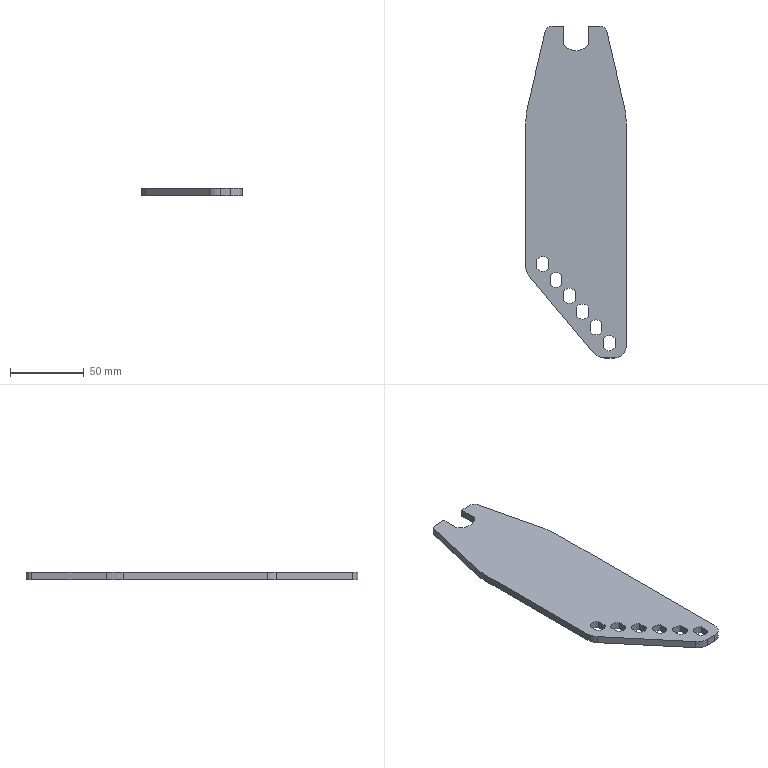Part | SolidWorks | features Fillet 5, ICE 5, Extrusion 1, LPattern 1 | 1 solid | 44 faces | box 68 x 225 x 5 mm | volume 61691 mm3 | plane 24 | cylinder 20 | commonest cylinder face diameters 10.1 x12 10 x2 20 x2 100 x2 16 x1 21 x1
STEP:
#1=CARTESIAN_POINT('',(-26.495,-51.96,5.));
#2=VERTEX_POINT('',#1);
#3=CARTESIAN_POINT('',(-18.495,-51.96,5.));
#4=VERTEX_POINT('',#3);
#5=CARTESIAN_POINT('',(-22.495,-48.877,5.));
#6=DIRECTION('',(0.,0.,1.));
#7=DIRECTION('',(1.,0.,0.));
#8=AXIS2_PLACEMENT_3D('',#5,#6,#7);
#9=CIRCLE('',#8,5.05);
#10=EDGE_CURVE('',#2,#4,#9,.T.);
#11=ORIENTED_EDGE('',*,*,#10,.T.);
#12=CARTESIAN_POINT('',(-18.495,-51.96,0.));
#13=VERTEX_POINT('',#12);
#14=CARTESIAN_POINT('',(-18.495,-51.96,0.));
#15=DIRECTION('',(0.,0.,1.));
#16=VECTOR('',#15,1000.);
#17=LINE('',#14,#16);
#18=EDGE_CURVE('',#13,#4,#17,.T.);
#19=ORIENTED_EDGE('',*,*,#18,.F.);
#20=CARTESIAN_POINT('',(-26.495,-51.96,0.));
#21=VERTEX_POINT('',#20);
#22=CARTESIAN_POINT('',(-22.495,-48.877,0.));
#23=DIRECTION('',(0.,0.,1.));
#24=DIRECTION('',(1.,0.,0.));
#25=AXIS2_PLACEMENT_3D('',#22,#23,#24);
#26=CIRCLE('',#25,5.05);
#27=EDGE_CURVE('',#21,#13,#26,.T.);
#28=ORIENTED_EDGE('',*,*,#27,.F.);
#29=CARTESIAN_POINT('',(-26.495,-51.96,0.));
#30=DIRECTION('',(0.,0.,1.));
#31=VECTOR('',#30,1000.);
#32=LINE('',#29,#31);
#33=EDGE_CURVE('',#21,#2,#32,.T.);
#34=ORIENTED_EDGE('',*,*,#33,.T.);
#35=EDGE_LOOP('',(#11,#19,#28,#34));
#36=FACE_OUTER_BOUND('',#35,.T.);
#37=CARTESIAN_POINT('',(-22.495,-48.877,-3.));
#38=DIRECTION('',(0.,0.,1.));
#39=DIRECTION('',(1.,0.,0.));
#40=AXIS2_PLACEMENT_3D('',#37,#38,#39);
#41=CYLINDRICAL_SURFACE('',#40,5.05);
#42=ADVANCED_FACE('',(#36),#41,.F.);
#43=CARTESIAN_POINT('',(-17.496,-62.684,5.));
#44=VERTEX_POINT('',#43);
#45=CARTESIAN_POINT('',(-9.496,-62.684,5.));
#46=VERTEX_POINT('',#45);
#47=CARTESIAN_POINT('',(-13.496,-59.602,5.));
#48=DIRECTION('',(0.,0.,1.));
#49=DIRECTION('',(1.,0.,0.));
#50=AXIS2_PLACEMENT_3D('',#47,#48,#49);
#51=CIRCLE('',#50,5.05);
#52=EDGE_CURVE('',#44,#46,#51,.T.);
#53=ORIENTED_EDGE('',*,*,#52,.T.);
#54=CARTESIAN_POINT('',(-9.496,-62.684,0.));
#55=VERTEX_POINT('',#54);
#56=CARTESIAN_POINT('',(-9.496,-62.684,0.));
#57=DIRECTION('',(0.,0.,1.));
#58=VECTOR('',#57,1000.);
#59=LINE('',#56,#58);
#60=EDGE_CURVE('',#55,#46,#59,.T.);
#61=ORIENTED_EDGE('',*,*,#60,.F.);
#62=CARTESIAN_POINT('',(-17.496,-62.684,0.));
#63=VERTEX_POINT('',#62);
#64=CARTESIAN_POINT('',(-13.496,-59.602,0.));
#65=DIRECTION('',(0.,0.,1.));
#66=DIRECTION('',(1.,0.,0.));
#67=AXIS2_PLACEMENT_3D('',#64,#65,#66);
#68=CIRCLE('',#67,5.05);
#69=EDGE_CURVE('',#63,#55,#68,.T.);
#70=ORIENTED_EDGE('',*,*,#69,.F.);
#71=CARTESIAN_POINT('',(-17.496,-62.684,0.));
#72=DIRECTION('',(0.,0.,1.));
#73=VECTOR('',#72,1000.);
#74=LINE('',#71,#73);
#75=EDGE_CURVE('',#63,#44,#74,.T.);
#76=ORIENTED_EDGE('',*,*,#75,.T.);
#77=EDGE_LOOP('',(#53,#61,#70,#76));
#78=FACE_OUTER_BOUND('',#77,.T.);
#79=CARTESIAN_POINT('',(-13.496,-59.602,-3.));
#80=DIRECTION('',(0.,0.,1.));
#81=DIRECTION('',(1.,0.,0.));
#82=AXIS2_PLACEMENT_3D('',#79,#80,#81);
#83=CYLINDRICAL_SURFACE('',#82,5.05);
#84=ADVANCED_FACE('',(#78),#83,.F.);
#85=CARTESIAN_POINT('',(-8.497,-73.409,5.));
#86=VERTEX_POINT('',#85);
#87=CARTESIAN_POINT('',(-0.4971,-73.409,5.));
#88=VERTEX_POINT('',#87);
#89=CARTESIAN_POINT('',(-4.497,-70.326,5.));
#90=DIRECTION('',(0.,0.,1.));
#91=DIRECTION('',(1.,0.,0.));
#92=AXIS2_PLACEMENT_3D('',#89,#90,#91);
#93=CIRCLE('',#92,5.05);
#94=EDGE_CURVE('',#86,#88,#93,.T.);
#95=ORIENTED_EDGE('',*,*,#94,.T.);
#96=CARTESIAN_POINT('',(-0.4971,-73.409,0.));
#97=VERTEX_POINT('',#96);
#98=CARTESIAN_POINT('',(-0.4971,-73.409,0.));
#99=DIRECTION('',(0.,0.,1.));
#100=VECTOR('',#99,1000.);
#101=LINE('',#98,#100);
#102=EDGE_CURVE('',#97,#88,#101,.T.);
#103=ORIENTED_EDGE('',*,*,#102,.F.);
#104=CARTESIAN_POINT('',(-8.497,-73.409,0.));
#105=VERTEX_POINT('',#104);
#106=CARTESIAN_POINT('',(-4.497,-70.326,0.));
#107=DIRECTION('',(0.,0.,1.));
#108=DIRECTION('',(1.,0.,0.));
#109=AXIS2_PLACEMENT_3D('',#106,#107,#108);
#110=CIRCLE('',#109,5.05);
#111=EDGE_CURVE('',#105,#97,#110,.T.);
#112=ORIENTED_EDGE('',*,*,#111,.F.);
#113=CARTESIAN_POINT('',(-8.497,-73.409,0.));
#114=DIRECTION('',(0.,0.,1.));
#115=VECTOR('',#114,1000.);
#116=LINE('',#113,#115);
#117=EDGE_CURVE('',#105,#86,#116,.T.);
#118=ORIENTED_EDGE('',*,*,#117,.T.);
#119=EDGE_LOOP('',(#95,#103,#112,#118));
#120=FACE_OUTER_BOUND('',#119,.T.);
#121=CARTESIAN_POINT('',(-4.497,-70.326,-3.));
#122=DIRECTION('',(0.,0.,1.));
#123=DIRECTION('',(1.,0.,0.));
#124=AXIS2_PLACEMENT_3D('',#121,#122,#123);
#125=CYLINDRICAL_SURFACE('',#124,5.05);
#126=ADVANCED_FACE('',(#120),#125,.F.);
#127=CARTESIAN_POINT('',(0.5019,-84.133,5.));
#128=VERTEX_POINT('',#127);
#129=CARTESIAN_POINT('',(8.502,-84.133,5.));
#130=VERTEX_POINT('',#129);
#131=CARTESIAN_POINT('',(4.502,-81.051,5.));
#132=DIRECTION('',(0.,0.,1.));
#133=DIRECTION('',(1.,0.,0.));
#134=AXIS2_PLACEMENT_3D('',#131,#132,#133);
#135=CIRCLE('',#134,5.05);
#136=EDGE_CURVE('',#128,#130,#135,.T.);
#137=ORIENTED_EDGE('',*,*,#136,.T.);
#138=CARTESIAN_POINT('',(8.502,-84.133,0.));
#139=VERTEX_POINT('',#138);
#140=CARTESIAN_POINT('',(8.502,-84.133,0.));
#141=DIRECTION('',(0.,0.,1.));
#142=VECTOR('',#141,1000.);
#143=LINE('',#140,#142);
#144=EDGE_CURVE('',#139,#130,#143,.T.);
#145=ORIENTED_EDGE('',*,*,#144,.F.);
#146=CARTESIAN_POINT('',(0.5019,-84.133,0.));
#147=VERTEX_POINT('',#146);
#148=CARTESIAN_POINT('',(4.502,-81.051,0.));
#149=DIRECTION('',(0.,0.,1.));
#150=DIRECTION('',(1.,0.,0.));
#151=AXIS2_PLACEMENT_3D('',#148,#149,#150);
#152=CIRCLE('',#151,5.05);
#153=EDGE_CURVE('',#147,#139,#152,.T.);
#154=ORIENTED_EDGE('',*,*,#153,.F.);
#155=CARTESIAN_POINT('',(0.5019,-84.133,0.));
#156=DIRECTION('',(0.,0.,1.));
#157=VECTOR('',#156,1000.);
#158=LINE('',#155,#157);
#159=EDGE_CURVE('',#147,#128,#158,.T.);
#160=ORIENTED_EDGE('',*,*,#159,.T.);
#161=EDGE_LOOP('',(#137,#145,#154,#160));
#162=FACE_OUTER_BOUND('',#161,.T.);
#163=CARTESIAN_POINT('',(4.502,-81.051,-3.));
#164=DIRECTION('',(0.,0.,1.));
#165=DIRECTION('',(1.,0.,0.));
#166=AXIS2_PLACEMENT_3D('',#163,#164,#165);
#167=CYLINDRICAL_SURFACE('',#166,5.05);
#168=ADVANCED_FACE('',(#162),#167,.F.);
#169=CARTESIAN_POINT('',(9.501,-94.858,5.));
#170=VERTEX_POINT('',#169);
#171=CARTESIAN_POINT('',(17.501,-94.858,5.));
#172=VERTEX_POINT('',#171);
#173=CARTESIAN_POINT('',(13.501,-91.775,5.));
#174=DIRECTION('',(0.,0.,1.));
#175=DIRECTION('',(1.,0.,0.));
#176=AXIS2_PLACEMENT_3D('',#173,#174,#175);
#177=CIRCLE('',#176,5.05);
#178=EDGE_CURVE('',#170,#172,#177,.T.);
#179=ORIENTED_EDGE('',*,*,#178,.T.);
#180=CARTESIAN_POINT('',(17.501,-94.858,0.));
#181=VERTEX_POINT('',#180);
#182=CARTESIAN_POINT('',(17.501,-94.858,0.));
#183=DIRECTION('',(0.,0.,1.));
#184=VECTOR('',#183,1000.);
#185=LINE('',#182,#184);
#186=EDGE_CURVE('',#181,#172,#185,.T.);
#187=ORIENTED_EDGE('',*,*,#186,.F.);
#188=CARTESIAN_POINT('',(9.501,-94.858,0.));
#189=VERTEX_POINT('',#188);
#190=CARTESIAN_POINT('',(13.501,-91.775,0.));
#191=DIRECTION('',(0.,0.,1.));
#192=DIRECTION('',(1.,0.,0.));
#193=AXIS2_PLACEMENT_3D('',#190,#191,#192);
#194=CIRCLE('',#193,5.05);
#195=EDGE_CURVE('',#189,#181,#194,.T.);
#196=ORIENTED_EDGE('',*,*,#195,.F.);
#197=CARTESIAN_POINT('',(9.501,-94.858,0.));
#198=DIRECTION('',(0.,0.,1.));
#199=VECTOR('',#198,1000.);
#200=LINE('',#197,#199);
#201=EDGE_CURVE('',#189,#170,#200,.T.);
#202=ORIENTED_EDGE('',*,*,#201,.T.);
#203=EDGE_LOOP('',(#179,#187,#196,#202));
#204=FACE_OUTER_BOUND('',#203,.T.);
#205=CARTESIAN_POINT('',(13.501,-91.775,-3.));
#206=DIRECTION('',(0.,0.,1.));
#207=DIRECTION('',(1.,0.,0.));
#208=AXIS2_PLACEMENT_3D('',#205,#206,#207);
#209=CYLINDRICAL_SURFACE('',#208,5.05);
#210=ADVANCED_FACE('',(#204),#209,.F.);
#211=CARTESIAN_POINT('',(18.5,-105.583,5.));
#212=VERTEX_POINT('',#211);
#213=CARTESIAN_POINT('',(26.5,-105.583,5.));
#214=VERTEX_POINT('',#213);
#215=CARTESIAN_POINT('',(22.5,-102.5,5.));
#216=DIRECTION('',(0.,0.,1.));
#217=DIRECTION('',(1.,0.,0.));
#218=AXIS2_PLACEMENT_3D('',#215,#216,#217);
#219=CIRCLE('',#218,5.05);
#220=EDGE_CURVE('',#212,#214,#219,.T.);
#221=ORIENTED_EDGE('',*,*,#220,.T.);
#222=CARTESIAN_POINT('',(26.5,-105.583,0.));
#223=VERTEX_POINT('',#222);
#224=CARTESIAN_POINT('',(26.5,-105.583,0.));
#225=DIRECTION('',(0.,0.,1.));
#226=VECTOR('',#225,1000.);
#227=LINE('',#224,#226);
#228=EDGE_CURVE('',#223,#214,#227,.T.);
#229=ORIENTED_EDGE('',*,*,#228,.F.);
#230=CARTESIAN_POINT('',(18.5,-105.583,0.));
#231=VERTEX_POINT('',#230);
#232=CARTESIAN_POINT('',(22.5,-102.5,0.));
#233=DIRECTION('',(0.,0.,1.));
#234=DIRECTION('',(1.,0.,0.));
#235=AXIS2_PLACEMENT_3D('',#232,#233,#234);
#236=CIRCLE('',#235,5.05);
#237=EDGE_CURVE('',#231,#223,#236,.T.);
#238=ORIENTED_EDGE('',*,*,#237,.F.);
#239=CARTESIAN_POINT('',(18.5,-105.583,0.));
#240=DIRECTION('',(0.,0.,1.));
#241=VECTOR('',#240,1000.);
#242=LINE('',#239,#241);
#243=EDGE_CURVE('',#231,#212,#242,.T.);
#244=ORIENTED_EDGE('',*,*,#243,.T.);
#245=EDGE_LOOP('',(#221,#229,#238,#244));
#246=FACE_OUTER_BOUND('',#245,.T.);
#247=CARTESIAN_POINT('',(22.5,-102.5,-3.));
#248=DIRECTION('',(0.,0.,1.));
#249=DIRECTION('',(1.,0.,0.));
#250=AXIS2_PLACEMENT_3D('',#247,#248,#249);
#251=CYLINDRICAL_SURFACE('',#250,5.05);
#252=ADVANCED_FACE('',(#246),#251,.F.);
#253=CARTESIAN_POINT('',(16.032,112.5,5.));
#254=VERTEX_POINT('',#253);
#255=CARTESIAN_POINT('',(8.5,112.5,5.));
#256=VERTEX_POINT('',#255);
#257=CARTESIAN_POINT('',(-34.,112.5,5.));
#258=DIRECTION('',(-1.,0.,0.));
#259=VECTOR('',#258,1000.);
#260=LINE('',#257,#259);
#261=EDGE_CURVE('',#254,#256,#260,.T.);
#262=ORIENTED_EDGE('',*,*,#261,.F.);
#263=CARTESIAN_POINT('',(16.032,112.5,0.));
#264=VERTEX_POINT('',#263);
#265=CARTESIAN_POINT('',(16.032,112.5,5.));
#266=DIRECTION('',(0.,0.,-1.));
#267=VECTOR('',#266,1000.);
#268=LINE('',#265,#267);
#269=EDGE_CURVE('',#254,#264,#268,.T.);
#270=ORIENTED_EDGE('',*,*,#269,.T.);
#271=CARTESIAN_POINT('',(8.5,112.5,0.));
#272=VERTEX_POINT('',#271);
#273=CARTESIAN_POINT('',(-34.,112.5,0.));
#274=DIRECTION('',(-1.,0.,0.));
#275=VECTOR('',#274,1000.);
#276=LINE('',#273,#275);
#277=EDGE_CURVE('',#264,#272,#276,.T.);
#278=ORIENTED_EDGE('',*,*,#277,.T.);
#279=CARTESIAN_POINT('',(8.5,112.5,-3.));
#280=DIRECTION('',(0.,0.,1.));
#281=VECTOR('',#280,1000.);
#282=LINE('',#279,#281);
#283=EDGE_CURVE('',#272,#256,#282,.T.);
#284=ORIENTED_EDGE('',*,*,#283,.T.);
#285=EDGE_LOOP('',(#262,#270,#278,#284));
#286=FACE_OUTER_BOUND('',#285,.T.);
#287=CARTESIAN_POINT('',(-34.,112.5,5.));
#288=DIRECTION('',(0.,-1.,0.));
#289=DIRECTION('',(0.,0.,-1.));
#290=AXIS2_PLACEMENT_3D('',#287,#288,#289);
#291=PLANE('',#290);
#292=ADVANCED_FACE('',(#286),#291,.F.);
#293=CARTESIAN_POINT('',(34.,-104.5,0.));
#294=VERTEX_POINT('',#293);
#295=CARTESIAN_POINT('',(34.,46.744,0.));
#296=VERTEX_POINT('',#295);
#297=CARTESIAN_POINT('',(34.,112.5,0.));
#298=DIRECTION('',(0.,1.,0.));
#299=VECTOR('',#298,1000.);
#300=LINE('',#297,#299);
#301=EDGE_CURVE('',#294,#296,#300,.T.);
#302=ORIENTED_EDGE('',*,*,#301,.T.);
#303=CARTESIAN_POINT('',(34.,46.744,5.));
#304=VERTEX_POINT('',#303);
#305=CARTESIAN_POINT('',(34.,46.744,5.));
#306=DIRECTION('',(0.,0.,1.));
#307=VECTOR('',#306,1000.);
#308=LINE('',#305,#307);
#309=EDGE_CURVE('',#296,#304,#308,.T.);
#310=ORIENTED_EDGE('',*,*,#309,.T.);
#311=CARTESIAN_POINT('',(34.,-104.5,5.));
#312=VERTEX_POINT('',#311);
#313=CARTESIAN_POINT('',(34.,112.5,5.));
#314=DIRECTION('',(0.,1.,0.));
#315=VECTOR('',#314,1000.);
#316=LINE('',#313,#315);
#317=EDGE_CURVE('',#312,#304,#316,.T.);
#318=ORIENTED_EDGE('',*,*,#317,.F.);
#319=CARTESIAN_POINT('',(34.,-104.5,5.));
#320=DIRECTION('',(0.,0.,-1.));
#321=VECTOR('',#320,1000.);
#322=LINE('',#319,#321);
#323=EDGE_CURVE('',#312,#294,#322,.T.);
#324=ORIENTED_EDGE('',*,*,#323,.T.);
#325=EDGE_LOOP('',(#302,#310,#318,#324));
#326=FACE_OUTER_BOUND('',#325,.T.);
#327=CARTESIAN_POINT('',(34.,112.5,5.));
#328=DIRECTION('',(-1.,0.,0.));
#329=DIRECTION('',(0.,-1.,0.));
#330=AXIS2_PLACEMENT_3D('',#327,#328,#329);
#331=PLANE('',#330);
#332=ADVANCED_FACE('',(#326),#331,.F.);
#333=CARTESIAN_POINT('',(-8.5,112.5,0.));
#334=VERTEX_POINT('',#333);
#335=CARTESIAN_POINT('',(-16.032,112.5,0.));
#336=VERTEX_POINT('',#335);
#337=CARTESIAN_POINT('',(-34.,112.5,0.));
#338=DIRECTION('',(-1.,0.,0.));
#339=VECTOR('',#338,1000.);
#340=LINE('',#337,#339);
#341=EDGE_CURVE('',#334,#336,#340,.T.);
#342=ORIENTED_EDGE('',*,*,#341,.T.);
#343=CARTESIAN_POINT('',(-16.032,112.5,5.));
#344=VERTEX_POINT('',#343);
#345=CARTESIAN_POINT('',(-16.032,112.5,5.));
#346=DIRECTION('',(0.,0.,1.));
#347=VECTOR('',#346,1000.);
#348=LINE('',#345,#347);
#349=EDGE_CURVE('',#336,#344,#348,.T.);
#350=ORIENTED_EDGE('',*,*,#349,.T.);
#351=CARTESIAN_POINT('',(-8.5,112.5,5.));
#352=VERTEX_POINT('',#351);
#353=CARTESIAN_POINT('',(-34.,112.5,5.));
#354=DIRECTION('',(-1.,0.,0.));
#355=VECTOR('',#354,1000.);
#356=LINE('',#353,#355);
#357=EDGE_CURVE('',#352,#344,#356,.T.);
#358=ORIENTED_EDGE('',*,*,#357,.F.);
#359=CARTESIAN_POINT('',(-8.5,112.5,-3.));
#360=DIRECTION('',(0.,0.,1.));
#361=VECTOR('',#360,1000.);
#362=LINE('',#359,#361);
#363=EDGE_CURVE('',#334,#352,#362,.T.);
#364=ORIENTED_EDGE('',*,*,#363,.F.);
#365=EDGE_LOOP('',(#342,#350,#358,#364));
#366=FACE_OUTER_BOUND('',#365,.T.);
#367=CARTESIAN_POINT('',(-34.,112.5,5.));
#368=DIRECTION('',(0.,-1.,0.));
#369=DIRECTION('',(0.,0.,-1.));
#370=AXIS2_PLACEMENT_3D('',#367,#368,#369);
#371=PLANE('',#370);
#372=ADVANCED_FACE('',(#366),#371,.F.);
#373=CARTESIAN_POINT('',(-34.,46.744,5.));
#374=VERTEX_POINT('',#373);
#375=CARTESIAN_POINT('',(-34.,-50.973,5.));
#376=VERTEX_POINT('',#375);
#377=CARTESIAN_POINT('',(-34.,112.5,5.));
#378=DIRECTION('',(0.,-1.,0.));
#379=VECTOR('',#378,1000.);
#380=LINE('',#377,#379);
#381=EDGE_CURVE('',#374,#376,#380,.T.);
#382=ORIENTED_EDGE('',*,*,#381,.F.);
#383=CARTESIAN_POINT('',(-34.,46.744,0.));
#384=VERTEX_POINT('',#383);
#385=CARTESIAN_POINT('',(-34.,46.744,5.));
#386=DIRECTION('',(0.,0.,-1.));
#387=VECTOR('',#386,1000.);
#388=LINE('',#385,#387);
#389=EDGE_CURVE('',#374,#384,#388,.T.);
#390=ORIENTED_EDGE('',*,*,#389,.T.);
#391=CARTESIAN_POINT('',(-34.,-50.973,0.));
#392=VERTEX_POINT('',#391);
#393=CARTESIAN_POINT('',(-34.,112.5,0.));
#394=DIRECTION('',(0.,-1.,0.));
#395=VECTOR('',#394,1000.);
#396=LINE('',#393,#395);
#397=EDGE_CURVE('',#384,#392,#396,.T.);
#398=ORIENTED_EDGE('',*,*,#397,.T.);
#399=CARTESIAN_POINT('',(-34.,-50.973,5.));
#400=DIRECTION('',(0.,0.,1.));
#401=VECTOR('',#400,1000.);
#402=LINE('',#399,#401);
#403=EDGE_CURVE('',#392,#376,#402,.T.);
#404=ORIENTED_EDGE('',*,*,#403,.T.);
#405=EDGE_LOOP('',(#382,#390,#398,#404));
#406=FACE_OUTER_BOUND('',#405,.T.);
#407=CARTESIAN_POINT('',(-34.,112.5,5.));
#408=DIRECTION('',(1.,0.,0.));
#409=DIRECTION('',(0.,1.,0.));
#410=AXIS2_PLACEMENT_3D('',#407,#408,#409);
#411=PLANE('',#410);
#412=ADVANCED_FACE('',(#406),#411,.F.);
#413=CARTESIAN_POINT('',(19.236,-112.5,5.));
#414=VERTEX_POINT('',#413);
#415=CARTESIAN_POINT('',(26.,-112.5,5.));
#416=VERTEX_POINT('',#415);
#417=CARTESIAN_POINT('',(-34.,-112.5,5.));
#418=DIRECTION('',(1.,0.,0.));
#419=VECTOR('',#418,1000.);
#420=LINE('',#417,#419);
#421=EDGE_CURVE('',#414,#416,#420,.T.);
#422=ORIENTED_EDGE('',*,*,#421,.F.);
#423=CARTESIAN_POINT('',(19.236,-112.5,0.));
#424=VERTEX_POINT('',#423);
#425=CARTESIAN_POINT('',(19.236,-112.5,5.));
#426=DIRECTION('',(0.,0.,-1.));
#427=VECTOR('',#426,1000.);
#428=LINE('',#425,#427);
#429=EDGE_CURVE('',#414,#424,#428,.T.);
#430=ORIENTED_EDGE('',*,*,#429,.T.);
#431=CARTESIAN_POINT('',(26.,-112.5,0.));
#432=VERTEX_POINT('',#431);
#433=CARTESIAN_POINT('',(-34.,-112.5,0.));
#434=DIRECTION('',(1.,0.,0.));
#435=VECTOR('',#434,1000.);
#436=LINE('',#433,#435);
#437=EDGE_CURVE('',#424,#432,#436,.T.);
#438=ORIENTED_EDGE('',*,*,#437,.T.);
#439=CARTESIAN_POINT('',(26.,-112.5,5.));
#440=DIRECTION('',(0.,0.,1.));
#441=VECTOR('',#440,1000.);
#442=LINE('',#439,#441);
#443=EDGE_CURVE('',#432,#416,#442,.T.);
#444=ORIENTED_EDGE('',*,*,#443,.T.);
#445=EDGE_LOOP('',(#422,#430,#438,#444));
#446=FACE_OUTER_BOUND('',#445,.T.);
#447=CARTESIAN_POINT('',(-34.,-112.5,5.));
#448=DIRECTION('',(0.,1.,0.));
#449=DIRECTION('',(0.,0.,1.));
#450=AXIS2_PLACEMENT_3D('',#447,#448,#449);
#451=PLANE('',#450);
#452=ADVANCED_FACE('',(#446),#451,.F.);
#453=ORIENTED_EDGE('',*,*,#317,.T.);
#454=CARTESIAN_POINT('',(32.692,58.105,5.));
#455=VERTEX_POINT('',#454);
#456=CARTESIAN_POINT('',(-16.,46.744,5.));
#457=DIRECTION('',(0.,0.,1.));
#458=DIRECTION('',(1.,0.,0.));
#459=AXIS2_PLACEMENT_3D('',#456,#457,#458);
#460=CIRCLE('',#459,50.);
#461=EDGE_CURVE('',#304,#455,#460,.T.);
#462=ORIENTED_EDGE('',*,*,#461,.T.);
#463=CARTESIAN_POINT('',(20.902,108.636,5.));
#464=VERTEX_POINT('',#463);
#465=CARTESIAN_POINT('',(20.,112.5,5.));
#466=DIRECTION('',(0.2272,-0.9738,0.));
#467=VECTOR('',#466,1000.);
#468=LINE('',#465,#467);
#469=EDGE_CURVE('',#464,#455,#468,.T.);
#470=ORIENTED_EDGE('',*,*,#469,.F.);
#471=CARTESIAN_POINT('',(16.032,107.5,5.));
#472=DIRECTION('',(0.,0.,1.));
#473=DIRECTION('',(1.,0.,0.));
#474=AXIS2_PLACEMENT_3D('',#471,#472,#473);
#475=CIRCLE('',#474,5.);
#476=EDGE_CURVE('',#464,#254,#475,.T.);
#477=ORIENTED_EDGE('',*,*,#476,.T.);
#478=ORIENTED_EDGE('',*,*,#261,.T.);
#479=CARTESIAN_POINT('',(8.5,100.171,5.));
#480=VERTEX_POINT('',#479);
#481=CARTESIAN_POINT('',(8.5,112.5,5.));
#482=DIRECTION('',(0.,1.,0.));
#483=VECTOR('',#482,1000.);
#484=LINE('',#481,#483);
#485=EDGE_CURVE('',#480,#256,#484,.T.);
#486=ORIENTED_EDGE('',*,*,#485,.F.);
#487=CARTESIAN_POINT('',(-8.5,100.171,5.));
#488=VERTEX_POINT('',#487);
#489=CARTESIAN_POINT('',(0.,106.336,5.));
#490=DIRECTION('',(0.,0.,1.));
#491=DIRECTION('',(1.,0.,0.));
#492=AXIS2_PLACEMENT_3D('',#489,#490,#491);
#493=CIRCLE('',#492,10.5);
#494=EDGE_CURVE('',#488,#480,#493,.T.);
#495=ORIENTED_EDGE('',*,*,#494,.F.);
#496=CARTESIAN_POINT('',(-8.5,112.5,5.));
#497=DIRECTION('',(0.,-1.,0.));
#498=VECTOR('',#497,1000.);
#499=LINE('',#496,#498);
#500=EDGE_CURVE('',#352,#488,#499,.T.);
#501=ORIENTED_EDGE('',*,*,#500,.F.);
#502=ORIENTED_EDGE('',*,*,#357,.T.);
#503=CARTESIAN_POINT('',(-20.902,108.636,5.));
#504=VERTEX_POINT('',#503);
#505=CARTESIAN_POINT('',(-16.032,107.5,5.));
#506=DIRECTION('',(0.,0.,1.));
#507=DIRECTION('',(1.,0.,0.));
#508=AXIS2_PLACEMENT_3D('',#505,#506,#507);
#509=CIRCLE('',#508,5.);
#510=EDGE_CURVE('',#344,#504,#509,.T.);
#511=ORIENTED_EDGE('',*,*,#510,.T.);
#512=CARTESIAN_POINT('',(-32.692,58.105,5.));
#513=VERTEX_POINT('',#512);
#514=CARTESIAN_POINT('',(-20.,112.5,5.));
#515=DIRECTION('',(0.2272,0.9738,0.));
#516=VECTOR('',#515,1000.);
#517=LINE('',#514,#516);
#518=EDGE_CURVE('',#513,#504,#517,.T.);
#519=ORIENTED_EDGE('',*,*,#518,.F.);
#520=CARTESIAN_POINT('',(16.,46.744,5.));
#521=DIRECTION('',(0.,0.,1.));
#522=DIRECTION('',(1.,0.,0.));
#523=AXIS2_PLACEMENT_3D('',#520,#521,#522);
#524=CIRCLE('',#523,50.);
#525=EDGE_CURVE('',#513,#374,#524,.T.);
#526=ORIENTED_EDGE('',*,*,#525,.T.);
#527=ORIENTED_EDGE('',*,*,#381,.T.);
#528=CARTESIAN_POINT('',(-31.66,-57.401,5.));
#529=VERTEX_POINT('',#528);
#530=CARTESIAN_POINT('',(-24.,-50.973,5.));
#531=DIRECTION('',(0.,0.,1.));
#532=DIRECTION('',(1.,0.,0.));
#533=AXIS2_PLACEMENT_3D('',#530,#531,#532);
#534=CIRCLE('',#533,10.);
#535=EDGE_CURVE('',#376,#529,#534,.T.);
#536=ORIENTED_EDGE('',*,*,#535,.T.);
#537=CARTESIAN_POINT('',(11.576,-108.928,5.));
#538=VERTEX_POINT('',#537);
#539=CARTESIAN_POINT('',(14.573,-112.5,5.));
#540=DIRECTION('',(-0.6428,0.766,0.));
#541=VECTOR('',#540,1000.);
#542=LINE('',#539,#541);
#543=EDGE_CURVE('',#538,#529,#542,.T.);
#544=ORIENTED_EDGE('',*,*,#543,.F.);
#545=CARTESIAN_POINT('',(19.236,-102.5,5.));
#546=DIRECTION('',(0.,0.,1.));
#547=DIRECTION('',(1.,0.,0.));
#548=AXIS2_PLACEMENT_3D('',#545,#546,#547);
#549=CIRCLE('',#548,10.);
#550=EDGE_CURVE('',#538,#414,#549,.T.);
#551=ORIENTED_EDGE('',*,*,#550,.T.);
#552=ORIENTED_EDGE('',*,*,#421,.T.);
#553=CARTESIAN_POINT('',(26.,-104.5,5.));
#554=DIRECTION('',(0.,0.,1.));
#555=DIRECTION('',(1.,0.,0.));
#556=AXIS2_PLACEMENT_3D('',#553,#554,#555);
#557=CIRCLE('',#556,8.);
#558=EDGE_CURVE('',#416,#312,#557,.T.);
#559=ORIENTED_EDGE('',*,*,#558,.T.);
#560=EDGE_LOOP('',(#453,#462,#470,#477,#478,#486,#495,#501,#502,#511,#519,#526,#527,#536,#544,#551,#552,#559));
#561=FACE_OUTER_BOUND('',#560,.T.);
#562=ORIENTED_EDGE('',*,*,#220,.F.);
#563=CARTESIAN_POINT('',(18.5,-99.417,5.));
#564=VERTEX_POINT('',#563);
#565=CARTESIAN_POINT('',(18.5,-105.583,5.));
#566=DIRECTION('',(0.,1.,0.));
#567=VECTOR('',#566,1000.);
#568=LINE('',#565,#567);
#569=EDGE_CURVE('',#212,#564,#568,.T.);
#570=ORIENTED_EDGE('',*,*,#569,.T.);
#571=CARTESIAN_POINT('',(26.5,-99.417,5.));
#572=VERTEX_POINT('',#571);
#573=CARTESIAN_POINT('',(22.5,-102.5,5.));
#574=DIRECTION('',(0.,0.,1.));
#575=DIRECTION('',(1.,0.,0.));
#576=AXIS2_PLACEMENT_3D('',#573,#574,#575);
#577=CIRCLE('',#576,5.05);
#578=EDGE_CURVE('',#572,#564,#577,.T.);
#579=ORIENTED_EDGE('',*,*,#578,.F.);
#580=CARTESIAN_POINT('',(26.5,-105.583,5.));
#581=DIRECTION('',(0.,-1.,0.));
#582=VECTOR('',#581,1000.);
#583=LINE('',#580,#582);
#584=EDGE_CURVE('',#572,#214,#583,.T.);
#585=ORIENTED_EDGE('',*,*,#584,.T.);
#586=EDGE_LOOP('',(#562,#570,#579,#585));
#587=FACE_BOUND('',#586,.T.);
#588=ORIENTED_EDGE('',*,*,#178,.F.);
#589=CARTESIAN_POINT('',(9.501,-88.693,5.));
#590=VERTEX_POINT('',#589);
#591=CARTESIAN_POINT('',(9.501,-94.858,5.));
#592=DIRECTION('',(0.,1.,0.));
#593=VECTOR('',#592,1000.);
#594=LINE('',#591,#593);
#595=EDGE_CURVE('',#170,#590,#594,.T.);
#596=ORIENTED_EDGE('',*,*,#595,.T.);
#597=CARTESIAN_POINT('',(17.501,-88.693,5.));
#598=VERTEX_POINT('',#597);
#599=CARTESIAN_POINT('',(13.501,-91.775,5.));
#600=DIRECTION('',(0.,0.,1.));
#601=DIRECTION('',(1.,0.,0.));
#602=AXIS2_PLACEMENT_3D('',#599,#600,#601);
#603=CIRCLE('',#602,5.05);
#604=EDGE_CURVE('',#598,#590,#603,.T.);
#605=ORIENTED_EDGE('',*,*,#604,.F.);
#606=CARTESIAN_POINT('',(17.501,-94.858,5.));
#607=DIRECTION('',(0.,-1.,0.));
#608=VECTOR('',#607,1000.);
#609=LINE('',#606,#608);
#610=EDGE_CURVE('',#598,#172,#609,.T.);
#611=ORIENTED_EDGE('',*,*,#610,.T.);
#612=EDGE_LOOP('',(#588,#596,#605,#611));
#613=FACE_BOUND('',#612,.T.);
#614=ORIENTED_EDGE('',*,*,#136,.F.);
#615=CARTESIAN_POINT('',(0.5019,-77.968,5.));
#616=VERTEX_POINT('',#615);
#617=CARTESIAN_POINT('',(0.5019,-84.133,5.));
#618=DIRECTION('',(0.,1.,0.));
#619=VECTOR('',#618,1000.);
#620=LINE('',#617,#619);
#621=EDGE_CURVE('',#128,#616,#620,.T.);
#622=ORIENTED_EDGE('',*,*,#621,.T.);
#623=CARTESIAN_POINT('',(8.502,-77.968,5.));
#624=VERTEX_POINT('',#623);
#625=CARTESIAN_POINT('',(4.502,-81.051,5.));
#626=DIRECTION('',(0.,0.,1.));
#627=DIRECTION('',(1.,0.,0.));
#628=AXIS2_PLACEMENT_3D('',#625,#626,#627);
#629=CIRCLE('',#628,5.05);
#630=EDGE_CURVE('',#624,#616,#629,.T.);
#631=ORIENTED_EDGE('',*,*,#630,.F.);
#632=CARTESIAN_POINT('',(8.502,-84.133,5.));
#633=DIRECTION('',(0.,-1.,0.));
#634=VECTOR('',#633,1000.);
#635=LINE('',#632,#634);
#636=EDGE_CURVE('',#624,#130,#635,.T.);
#637=ORIENTED_EDGE('',*,*,#636,.T.);
#638=EDGE_LOOP('',(#614,#622,#631,#637));
#639=FACE_BOUND('',#638,.T.);
#640=ORIENTED_EDGE('',*,*,#94,.F.);
#641=CARTESIAN_POINT('',(-8.497,-67.244,5.));
#642=VERTEX_POINT('',#641);
#643=CARTESIAN_POINT('',(-8.497,-73.409,5.));
#644=DIRECTION('',(0.,1.,0.));
#645=VECTOR('',#644,1000.);
#646=LINE('',#643,#645);
#647=EDGE_CURVE('',#86,#642,#646,.T.);
#648=ORIENTED_EDGE('',*,*,#647,.T.);
#649=CARTESIAN_POINT('',(-0.4971,-67.244,5.));
#650=VERTEX_POINT('',#649);
#651=CARTESIAN_POINT('',(-4.497,-70.326,5.));
#652=DIRECTION('',(0.,0.,1.));
#653=DIRECTION('',(1.,0.,0.));
#654=AXIS2_PLACEMENT_3D('',#651,#652,#653);
#655=CIRCLE('',#654,5.05);
#656=EDGE_CURVE('',#650,#642,#655,.T.);
#657=ORIENTED_EDGE('',*,*,#656,.F.);
#658=CARTESIAN_POINT('',(-0.4971,-73.409,5.));
#659=DIRECTION('',(0.,-1.,0.));
#660=VECTOR('',#659,1000.);
#661=LINE('',#658,#660);
#662=EDGE_CURVE('',#650,#88,#661,.T.);
#663=ORIENTED_EDGE('',*,*,#662,.T.);
#664=EDGE_LOOP('',(#640,#648,#657,#663));
#665=FACE_BOUND('',#664,.T.);
#666=ORIENTED_EDGE('',*,*,#52,.F.);
#667=CARTESIAN_POINT('',(-17.496,-56.519,5.));
#668=VERTEX_POINT('',#667);
#669=CARTESIAN_POINT('',(-17.496,-62.684,5.));
#670=DIRECTION('',(0.,1.,0.));
#671=VECTOR('',#670,1000.);
#672=LINE('',#669,#671);
#673=EDGE_CURVE('',#44,#668,#672,.T.);
#674=ORIENTED_EDGE('',*,*,#673,.T.);
#675=CARTESIAN_POINT('',(-9.496,-56.519,5.));
#676=VERTEX_POINT('',#675);
#677=CARTESIAN_POINT('',(-13.496,-59.602,5.));
#678=DIRECTION('',(0.,0.,1.));
#679=DIRECTION('',(1.,0.,0.));
#680=AXIS2_PLACEMENT_3D('',#677,#678,#679);
#681=CIRCLE('',#680,5.05);
#682=EDGE_CURVE('',#676,#668,#681,.T.);
#683=ORIENTED_EDGE('',*,*,#682,.F.);
#684=CARTESIAN_POINT('',(-9.496,-62.684,5.));
#685=DIRECTION('',(0.,-1.,0.));
#686=VECTOR('',#685,1000.);
#687=LINE('',#684,#686);
#688=EDGE_CURVE('',#676,#46,#687,.T.);
#689=ORIENTED_EDGE('',*,*,#688,.T.);
#690=EDGE_LOOP('',(#666,#674,#683,#689));
#691=FACE_BOUND('',#690,.T.);
#692=ORIENTED_EDGE('',*,*,#10,.F.);
#693=CARTESIAN_POINT('',(-26.495,-45.794,5.));
#694=VERTEX_POINT('',#693);
#695=CARTESIAN_POINT('',(-26.495,-51.96,5.));
#696=DIRECTION('',(0.,1.,0.));
#697=VECTOR('',#696,1000.);
#698=LINE('',#695,#697);
#699=EDGE_CURVE('',#2,#694,#698,.T.);
#700=ORIENTED_EDGE('',*,*,#699,.T.);
#701=CARTESIAN_POINT('',(-18.495,-45.794,5.));
#702=VERTEX_POINT('',#701);
#703=CARTESIAN_POINT('',(-22.495,-48.877,5.));
#704=DIRECTION('',(0.,0.,1.));
#705=DIRECTION('',(1.,0.,0.));
#706=AXIS2_PLACEMENT_3D('',#703,#704,#705);
#707=CIRCLE('',#706,5.05);
#708=EDGE_CURVE('',#702,#694,#707,.T.);
#709=ORIENTED_EDGE('',*,*,#708,.F.);
#710=CARTESIAN_POINT('',(-18.495,-51.96,5.));
#711=DIRECTION('',(0.,-1.,0.));
#712=VECTOR('',#711,1000.);
#713=LINE('',#710,#712);
#714=EDGE_CURVE('',#702,#4,#713,.T.);
#715=ORIENTED_EDGE('',*,*,#714,.T.);
#716=EDGE_LOOP('',(#692,#700,#709,#715));
#717=FACE_BOUND('',#716,.T.);
#718=CARTESIAN_POINT('',(0.,0.,5.));
#719=DIRECTION('',(0.,0.,1.));
#720=DIRECTION('',(1.,0.,0.));
#721=AXIS2_PLACEMENT_3D('',#718,#719,#720);
#722=PLANE('',#721);
#723=ADVANCED_FACE('',(#561,#587,#613,#639,#665,#691,#717),#722,.T.);
#724=ORIENTED_EDGE('',*,*,#237,.T.);
#725=CARTESIAN_POINT('',(26.5,-99.417,0.));
#726=VERTEX_POINT('',#725);
#727=CARTESIAN_POINT('',(26.5,-105.583,0.));
#728=DIRECTION('',(0.,-1.,0.));
#729=VECTOR('',#728,1000.);
#730=LINE('',#727,#729);
#731=EDGE_CURVE('',#726,#223,#730,.T.);
#732=ORIENTED_EDGE('',*,*,#731,.F.);
#733=CARTESIAN_POINT('',(18.5,-99.417,0.));
#734=VERTEX_POINT('',#733);
#735=CARTESIAN_POINT('',(22.5,-102.5,0.));
#736=DIRECTION('',(0.,0.,1.));
#737=DIRECTION('',(1.,0.,0.));
#738=AXIS2_PLACEMENT_3D('',#735,#736,#737);
#739=CIRCLE('',#738,5.05);
#740=EDGE_CURVE('',#726,#734,#739,.T.);
#741=ORIENTED_EDGE('',*,*,#740,.T.);
#742=CARTESIAN_POINT('',(18.5,-105.583,0.));
#743=DIRECTION('',(0.,1.,0.));
#744=VECTOR('',#743,1000.);
#745=LINE('',#742,#744);
#746=EDGE_CURVE('',#231,#734,#745,.T.);
#747=ORIENTED_EDGE('',*,*,#746,.F.);
#748=EDGE_LOOP('',(#724,#732,#741,#747));
#749=FACE_BOUND('',#748,.T.);
#750=ORIENTED_EDGE('',*,*,#195,.T.);
#751=CARTESIAN_POINT('',(17.501,-88.693,0.));
#752=VERTEX_POINT('',#751);
#753=CARTESIAN_POINT('',(17.501,-94.858,0.));
#754=DIRECTION('',(0.,-1.,0.));
#755=VECTOR('',#754,1000.);
#756=LINE('',#753,#755);
#757=EDGE_CURVE('',#752,#181,#756,.T.);
#758=ORIENTED_EDGE('',*,*,#757,.F.);
#759=CARTESIAN_POINT('',(9.501,-88.693,0.));
#760=VERTEX_POINT('',#759);
#761=CARTESIAN_POINT('',(13.501,-91.775,0.));
#762=DIRECTION('',(0.,0.,1.));
#763=DIRECTION('',(1.,0.,0.));
#764=AXIS2_PLACEMENT_3D('',#761,#762,#763);
#765=CIRCLE('',#764,5.05);
#766=EDGE_CURVE('',#752,#760,#765,.T.);
#767=ORIENTED_EDGE('',*,*,#766,.T.);
#768=CARTESIAN_POINT('',(9.501,-94.858,0.));
#769=DIRECTION('',(0.,1.,0.));
#770=VECTOR('',#769,1000.);
#771=LINE('',#768,#770);
#772=EDGE_CURVE('',#189,#760,#771,.T.);
#773=ORIENTED_EDGE('',*,*,#772,.F.);
#774=EDGE_LOOP('',(#750,#758,#767,#773));
#775=FACE_BOUND('',#774,.T.);
#776=ORIENTED_EDGE('',*,*,#153,.T.);
#777=CARTESIAN_POINT('',(8.502,-77.968,0.));
#778=VERTEX_POINT('',#777);
#779=CARTESIAN_POINT('',(8.502,-84.133,0.));
#780=DIRECTION('',(0.,-1.,0.));
#781=VECTOR('',#780,1000.);
#782=LINE('',#779,#781);
#783=EDGE_CURVE('',#778,#139,#782,.T.);
#784=ORIENTED_EDGE('',*,*,#783,.F.);
#785=CARTESIAN_POINT('',(0.5019,-77.968,0.));
#786=VERTEX_POINT('',#785);
#787=CARTESIAN_POINT('',(4.502,-81.051,0.));
#788=DIRECTION('',(0.,0.,1.));
#789=DIRECTION('',(1.,0.,0.));
#790=AXIS2_PLACEMENT_3D('',#787,#788,#789);
#791=CIRCLE('',#790,5.05);
#792=EDGE_CURVE('',#778,#786,#791,.T.);
#793=ORIENTED_EDGE('',*,*,#792,.T.);
#794=CARTESIAN_POINT('',(0.5019,-84.133,0.));
#795=DIRECTION('',(0.,1.,0.));
#796=VECTOR('',#795,1000.);
#797=LINE('',#794,#796);
#798=EDGE_CURVE('',#147,#786,#797,.T.);
#799=ORIENTED_EDGE('',*,*,#798,.F.);
#800=EDGE_LOOP('',(#776,#784,#793,#799));
#801=FACE_BOUND('',#800,.T.);
#802=ORIENTED_EDGE('',*,*,#111,.T.);
#803=CARTESIAN_POINT('',(-0.4971,-67.244,0.));
#804=VERTEX_POINT('',#803);
#805=CARTESIAN_POINT('',(-0.4971,-73.409,0.));
#806=DIRECTION('',(0.,-1.,0.));
#807=VECTOR('',#806,1000.);
#808=LINE('',#805,#807);
#809=EDGE_CURVE('',#804,#97,#808,.T.);
#810=ORIENTED_EDGE('',*,*,#809,.F.);
#811=CARTESIAN_POINT('',(-8.497,-67.244,0.));
#812=VERTEX_POINT('',#811);
#813=CARTESIAN_POINT('',(-4.497,-70.326,0.));
#814=DIRECTION('',(0.,0.,1.));
#815=DIRECTION('',(1.,0.,0.));
#816=AXIS2_PLACEMENT_3D('',#813,#814,#815);
#817=CIRCLE('',#816,5.05);
#818=EDGE_CURVE('',#804,#812,#817,.T.);
#819=ORIENTED_EDGE('',*,*,#818,.T.);
#820=CARTESIAN_POINT('',(-8.497,-73.409,0.));
#821=DIRECTION('',(0.,1.,0.));
#822=VECTOR('',#821,1000.);
#823=LINE('',#820,#822);
#824=EDGE_CURVE('',#105,#812,#823,.T.);
#825=ORIENTED_EDGE('',*,*,#824,.F.);
#826=EDGE_LOOP('',(#802,#810,#819,#825));
#827=FACE_BOUND('',#826,.T.);
#828=ORIENTED_EDGE('',*,*,#69,.T.);
#829=CARTESIAN_POINT('',(-9.496,-56.519,0.));
#830=VERTEX_POINT('',#829);
#831=CARTESIAN_POINT('',(-9.496,-62.684,0.));
#832=DIRECTION('',(0.,-1.,0.));
#833=VECTOR('',#832,1000.);
#834=LINE('',#831,#833);
#835=EDGE_CURVE('',#830,#55,#834,.T.);
#836=ORIENTED_EDGE('',*,*,#835,.F.);
#837=CARTESIAN_POINT('',(-17.496,-56.519,0.));
#838=VERTEX_POINT('',#837);
#839=CARTESIAN_POINT('',(-13.496,-59.602,0.));
#840=DIRECTION('',(0.,0.,1.));
#841=DIRECTION('',(1.,0.,0.));
#842=AXIS2_PLACEMENT_3D('',#839,#840,#841);
#843=CIRCLE('',#842,5.05);
#844=EDGE_CURVE('',#830,#838,#843,.T.);
#845=ORIENTED_EDGE('',*,*,#844,.T.);
#846=CARTESIAN_POINT('',(-17.496,-62.684,0.));
#847=DIRECTION('',(0.,1.,0.));
#848=VECTOR('',#847,1000.);
#849=LINE('',#846,#848);
#850=EDGE_CURVE('',#63,#838,#849,.T.);
#851=ORIENTED_EDGE('',*,*,#850,.F.);
#852=EDGE_LOOP('',(#828,#836,#845,#851));
#853=FACE_BOUND('',#852,.T.);
#854=ORIENTED_EDGE('',*,*,#27,.T.);
#855=CARTESIAN_POINT('',(-18.495,-45.794,0.));
#856=VERTEX_POINT('',#855);
#857=CARTESIAN_POINT('',(-18.495,-51.96,0.));
#858=DIRECTION('',(0.,-1.,0.));
#859=VECTOR('',#858,1000.);
#860=LINE('',#857,#859);
#861=EDGE_CURVE('',#856,#13,#860,.T.);
#862=ORIENTED_EDGE('',*,*,#861,.F.);
#863=CARTESIAN_POINT('',(-26.495,-45.794,0.));
#864=VERTEX_POINT('',#863);
#865=CARTESIAN_POINT('',(-22.495,-48.877,0.));
#866=DIRECTION('',(0.,0.,1.));
#867=DIRECTION('',(1.,0.,0.));
#868=AXIS2_PLACEMENT_3D('',#865,#866,#867);
#869=CIRCLE('',#868,5.05);
#870=EDGE_CURVE('',#856,#864,#869,.T.);
#871=ORIENTED_EDGE('',*,*,#870,.T.);
#872=CARTESIAN_POINT('',(-26.495,-51.96,0.));
#873=DIRECTION('',(0.,1.,0.));
#874=VECTOR('',#873,1000.);
#875=LINE('',#872,#874);
#876=EDGE_CURVE('',#21,#864,#875,.T.);
#877=ORIENTED_EDGE('',*,*,#876,.F.);
#878=EDGE_LOOP('',(#854,#862,#871,#877));
#879=FACE_BOUND('',#878,.T.);
#880=CARTESIAN_POINT('',(20.902,108.636,0.));
#881=VERTEX_POINT('',#880);
#882=CARTESIAN_POINT('',(32.692,58.105,0.));
#883=VERTEX_POINT('',#882);
#884=CARTESIAN_POINT('',(20.,112.5,0.));
#885=DIRECTION('',(0.2272,-0.9738,0.));
#886=VECTOR('',#885,1000.);
#887=LINE('',#884,#886);
#888=EDGE_CURVE('',#881,#883,#887,.T.);
#889=ORIENTED_EDGE('',*,*,#888,.T.);
#890=CARTESIAN_POINT('',(-16.,46.744,0.));
#891=DIRECTION('',(0.,0.,-1.));
#892=DIRECTION('',(1.,0.,0.));
#893=AXIS2_PLACEMENT_3D('',#890,#891,#892);
#894=CIRCLE('',#893,50.);
#895=EDGE_CURVE('',#883,#296,#894,.T.);
#896=ORIENTED_EDGE('',*,*,#895,.T.);
#897=ORIENTED_EDGE('',*,*,#301,.F.);
#898=CARTESIAN_POINT('',(26.,-104.5,0.));
#899=DIRECTION('',(0.,0.,-1.));
#900=DIRECTION('',(1.,0.,0.));
#901=AXIS2_PLACEMENT_3D('',#898,#899,#900);
#902=CIRCLE('',#901,8.);
#903=EDGE_CURVE('',#294,#432,#902,.T.);
#904=ORIENTED_EDGE('',*,*,#903,.T.);
#905=ORIENTED_EDGE('',*,*,#437,.F.);
#906=CARTESIAN_POINT('',(11.576,-108.928,0.));
#907=VERTEX_POINT('',#906);
#908=CARTESIAN_POINT('',(19.236,-102.5,0.));
#909=DIRECTION('',(0.,0.,-1.));
#910=DIRECTION('',(1.,0.,0.));
#911=AXIS2_PLACEMENT_3D('',#908,#909,#910);
#912=CIRCLE('',#911,10.);
#913=EDGE_CURVE('',#424,#907,#912,.T.);
#914=ORIENTED_EDGE('',*,*,#913,.T.);
#915=CARTESIAN_POINT('',(-31.66,-57.401,0.));
#916=VERTEX_POINT('',#915);
#917=CARTESIAN_POINT('',(14.573,-112.5,0.));
#918=DIRECTION('',(-0.6428,0.766,0.));
#919=VECTOR('',#918,1000.);
#920=LINE('',#917,#919);
#921=EDGE_CURVE('',#907,#916,#920,.T.);
#922=ORIENTED_EDGE('',*,*,#921,.T.);
#923=CARTESIAN_POINT('',(-24.,-50.973,0.));
#924=DIRECTION('',(0.,0.,-1.));
#925=DIRECTION('',(1.,0.,0.));
#926=AXIS2_PLACEMENT_3D('',#923,#924,#925);
#927=CIRCLE('',#926,10.);
#928=EDGE_CURVE('',#916,#392,#927,.T.);
#929=ORIENTED_EDGE('',*,*,#928,.T.);
#930=ORIENTED_EDGE('',*,*,#397,.F.);
#931=CARTESIAN_POINT('',(-32.692,58.105,0.));
#932=VERTEX_POINT('',#931);
#933=CARTESIAN_POINT('',(16.,46.744,0.));
#934=DIRECTION('',(0.,0.,-1.));
#935=DIRECTION('',(1.,0.,0.));
#936=AXIS2_PLACEMENT_3D('',#933,#934,#935);
#937=CIRCLE('',#936,50.);
#938=EDGE_CURVE('',#384,#932,#937,.T.);
#939=ORIENTED_EDGE('',*,*,#938,.T.);
#940=CARTESIAN_POINT('',(-20.902,108.636,0.));
#941=VERTEX_POINT('',#940);
#942=CARTESIAN_POINT('',(-20.,112.5,0.));
#943=DIRECTION('',(0.2272,0.9738,0.));
#944=VECTOR('',#943,1000.);
#945=LINE('',#942,#944);
#946=EDGE_CURVE('',#932,#941,#945,.T.);
#947=ORIENTED_EDGE('',*,*,#946,.T.);
#948=CARTESIAN_POINT('',(-16.032,107.5,0.));
#949=DIRECTION('',(0.,0.,-1.));
#950=DIRECTION('',(1.,0.,0.));
#951=AXIS2_PLACEMENT_3D('',#948,#949,#950);
#952=CIRCLE('',#951,5.);
#953=EDGE_CURVE('',#941,#336,#952,.T.);
#954=ORIENTED_EDGE('',*,*,#953,.T.);
#955=ORIENTED_EDGE('',*,*,#341,.F.);
#956=CARTESIAN_POINT('',(-8.5,100.171,0.));
#957=VERTEX_POINT('',#956);
#958=CARTESIAN_POINT('',(-8.5,0.,0.));
#959=DIRECTION('',(0.,-1.,0.));
#960=VECTOR('',#959,1000.);
#961=LINE('',#958,#960);
#962=EDGE_CURVE('',#334,#957,#961,.T.);
#963=ORIENTED_EDGE('',*,*,#962,.T.);
#964=CARTESIAN_POINT('',(8.5,100.171,0.));
#965=VERTEX_POINT('',#964);
#966=CARTESIAN_POINT('',(0.,106.336,0.));
#967=DIRECTION('',(0.,0.,1.));
#968=DIRECTION('',(1.,0.,0.));
#969=AXIS2_PLACEMENT_3D('',#966,#967,#968);
#970=CIRCLE('',#969,10.5);
#971=EDGE_CURVE('',#957,#965,#970,.T.);
#972=ORIENTED_EDGE('',*,*,#971,.T.);
#973=CARTESIAN_POINT('',(8.5,0.,0.));
#974=DIRECTION('',(0.,1.,0.));
#975=VECTOR('',#974,1000.);
#976=LINE('',#973,#975);
#977=EDGE_CURVE('',#965,#272,#976,.T.);
#978=ORIENTED_EDGE('',*,*,#977,.T.);
#979=ORIENTED_EDGE('',*,*,#277,.F.);
#980=CARTESIAN_POINT('',(16.032,107.5,0.));
#981=DIRECTION('',(0.,0.,-1.));
#982=DIRECTION('',(1.,0.,0.));
#983=AXIS2_PLACEMENT_3D('',#980,#981,#982);
#984=CIRCLE('',#983,5.);
#985=EDGE_CURVE('',#264,#881,#984,.T.);
#986=ORIENTED_EDGE('',*,*,#985,.T.);
#987=EDGE_LOOP('',(#889,#896,#897,#904,#905,#914,#922,#929,#930,#939,#947,#954,#955,#963,#972,#978,#979,#986));
#988=FACE_OUTER_BOUND('',#987,.T.);
#989=CARTESIAN_POINT('',(0.,0.,0.));
#990=DIRECTION('',(0.,0.,1.));
#991=DIRECTION('',(1.,0.,0.));
#992=AXIS2_PLACEMENT_3D('',#989,#990,#991);
#993=PLANE('',#992);
#994=ADVANCED_FACE('',(#749,#775,#801,#827,#853,#879,#988),#993,.F.);
#995=ORIENTED_EDGE('',*,*,#870,.F.);
#996=CARTESIAN_POINT('',(-18.495,-45.794,0.));
#997=DIRECTION('',(0.,0.,1.));
#998=VECTOR('',#997,1000.);
#999=LINE('',#996,#998);
#1000=EDGE_CURVE('',#856,#702,#999,.T.);
#1001=ORIENTED_EDGE('',*,*,#1000,.T.);
#1002=ORIENTED_EDGE('',*,*,#708,.T.);
#1003=CARTESIAN_POINT('',(-26.495,-45.794,0.));
#1004=DIRECTION('',(0.,0.,1.));
#1005=VECTOR('',#1004,1000.);
#1006=LINE('',#1003,#1005);
#1007=EDGE_CURVE('',#864,#694,#1006,.T.);
#1008=ORIENTED_EDGE('',*,*,#1007,.F.);
#1009=EDGE_LOOP('',(#995,#1001,#1002,#1008));
#1010=FACE_OUTER_BOUND('',#1009,.T.);
#1011=CARTESIAN_POINT('',(-22.495,-48.877,-3.));
#1012=DIRECTION('',(0.,0.,1.));
#1013=DIRECTION('',(1.,0.,0.));
#1014=AXIS2_PLACEMENT_3D('',#1011,#1012,#1013);
#1015=CYLINDRICAL_SURFACE('',#1014,5.05);
#1016=ADVANCED_FACE('',(#1010),#1015,.F.);
#1017=ORIENTED_EDGE('',*,*,#844,.F.);
#1018=CARTESIAN_POINT('',(-9.496,-56.519,0.));
#1019=DIRECTION('',(0.,0.,1.));
#1020=VECTOR('',#1019,1000.);
#1021=LINE('',#1018,#1020);
#1022=EDGE_CURVE('',#830,#676,#1021,.T.);
#1023=ORIENTED_EDGE('',*,*,#1022,.T.);
#1024=ORIENTED_EDGE('',*,*,#682,.T.);
#1025=CARTESIAN_POINT('',(-17.496,-56.519,0.));
#1026=DIRECTION('',(0.,0.,1.));
#1027=VECTOR('',#1026,1000.);
#1028=LINE('',#1025,#1027);
#1029=EDGE_CURVE('',#838,#668,#1028,.T.);
#1030=ORIENTED_EDGE('',*,*,#1029,.F.);
#1031=EDGE_LOOP('',(#1017,#1023,#1024,#1030));
#1032=FACE_OUTER_BOUND('',#1031,.T.);
#1033=CARTESIAN_POINT('',(-13.496,-59.602,-3.));
#1034=DIRECTION('',(0.,0.,1.));
#1035=DIRECTION('',(1.,0.,0.));
#1036=AXIS2_PLACEMENT_3D('',#1033,#1034,#1035);
#1037=CYLINDRICAL_SURFACE('',#1036,5.05);
#1038=ADVANCED_FACE('',(#1032),#1037,.F.);
#1039=ORIENTED_EDGE('',*,*,#818,.F.);
#1040=CARTESIAN_POINT('',(-0.4971,-67.244,0.));
#1041=DIRECTION('',(0.,0.,1.));
#1042=VECTOR('',#1041,1000.);
#1043=LINE('',#1040,#1042);
#1044=EDGE_CURVE('',#804,#650,#1043,.T.);
#1045=ORIENTED_EDGE('',*,*,#1044,.T.);
#1046=ORIENTED_EDGE('',*,*,#656,.T.);
#1047=CARTESIAN_POINT('',(-8.497,-67.244,0.));
#1048=DIRECTION('',(0.,0.,1.));
#1049=VECTOR('',#1048,1000.);
#1050=LINE('',#1047,#1049);
#1051=EDGE_CURVE('',#812,#642,#1050,.T.);
#1052=ORIENTED_EDGE('',*,*,#1051,.F.);
#1053=EDGE_LOOP('',(#1039,#1045,#1046,#1052));
#1054=FACE_OUTER_BOUND('',#1053,.T.);
#1055=CARTESIAN_POINT('',(-4.497,-70.326,-3.));
#1056=DIRECTION('',(0.,0.,1.));
#1057=DIRECTION('',(1.,0.,0.));
#1058=AXIS2_PLACEMENT_3D('',#1055,#1056,#1057);
#1059=CYLINDRICAL_SURFACE('',#1058,5.05);
#1060=ADVANCED_FACE('',(#1054),#1059,.F.);
#1061=ORIENTED_EDGE('',*,*,#792,.F.);
#1062=CARTESIAN_POINT('',(8.502,-77.968,0.));
#1063=DIRECTION('',(0.,0.,1.));
#1064=VECTOR('',#1063,1000.);
#1065=LINE('',#1062,#1064);
#1066=EDGE_CURVE('',#778,#624,#1065,.T.);
#1067=ORIENTED_EDGE('',*,*,#1066,.T.);
#1068=ORIENTED_EDGE('',*,*,#630,.T.);
#1069=CARTESIAN_POINT('',(0.5019,-77.968,0.));
#1070=DIRECTION('',(0.,0.,1.));
#1071=VECTOR('',#1070,1000.);
#1072=LINE('',#1069,#1071);
#1073=EDGE_CURVE('',#786,#616,#1072,.T.);
#1074=ORIENTED_EDGE('',*,*,#1073,.F.);
#1075=EDGE_LOOP('',(#1061,#1067,#1068,#1074));
#1076=FACE_OUTER_BOUND('',#1075,.T.);
#1077=CARTESIAN_POINT('',(4.502,-81.051,-3.));
#1078=DIRECTION('',(0.,0.,1.));
#1079=DIRECTION('',(1.,0.,0.));
#1080=AXIS2_PLACEMENT_3D('',#1077,#1078,#1079);
#1081=CYLINDRICAL_SURFACE('',#1080,5.05);
#1082=ADVANCED_FACE('',(#1076),#1081,.F.);
#1083=ORIENTED_EDGE('',*,*,#766,.F.);
#1084=CARTESIAN_POINT('',(17.501,-88.693,0.));
#1085=DIRECTION('',(0.,0.,1.));
#1086=VECTOR('',#1085,1000.);
#1087=LINE('',#1084,#1086);
#1088=EDGE_CURVE('',#752,#598,#1087,.T.);
#1089=ORIENTED_EDGE('',*,*,#1088,.T.);
#1090=ORIENTED_EDGE('',*,*,#604,.T.);
#1091=CARTESIAN_POINT('',(9.501,-88.693,0.));
#1092=DIRECTION('',(0.,0.,1.));
#1093=VECTOR('',#1092,1000.);
#1094=LINE('',#1091,#1093);
#1095=EDGE_CURVE('',#760,#590,#1094,.T.);
#1096=ORIENTED_EDGE('',*,*,#1095,.F.);
#1097=EDGE_LOOP('',(#1083,#1089,#1090,#1096));
#1098=FACE_OUTER_BOUND('',#1097,.T.);
#1099=CARTESIAN_POINT('',(13.501,-91.775,-3.));
#1100=DIRECTION('',(0.,0.,1.));
#1101=DIRECTION('',(1.,0.,0.));
#1102=AXIS2_PLACEMENT_3D('',#1099,#1100,#1101);
#1103=CYLINDRICAL_SURFACE('',#1102,5.05);
#1104=ADVANCED_FACE('',(#1098),#1103,.F.);
#1105=ORIENTED_EDGE('',*,*,#740,.F.);
#1106=CARTESIAN_POINT('',(26.5,-99.417,0.));
#1107=DIRECTION('',(0.,0.,1.));
#1108=VECTOR('',#1107,1000.);
#1109=LINE('',#1106,#1108);
#1110=EDGE_CURVE('',#726,#572,#1109,.T.);
#1111=ORIENTED_EDGE('',*,*,#1110,.T.);
#1112=ORIENTED_EDGE('',*,*,#578,.T.);
#1113=CARTESIAN_POINT('',(18.5,-99.417,0.));
#1114=DIRECTION('',(0.,0.,1.));
#1115=VECTOR('',#1114,1000.);
#1116=LINE('',#1113,#1115);
#1117=EDGE_CURVE('',#734,#564,#1116,.T.);
#1118=ORIENTED_EDGE('',*,*,#1117,.F.);
#1119=EDGE_LOOP('',(#1105,#1111,#1112,#1118));
#1120=FACE_OUTER_BOUND('',#1119,.T.);
#1121=CARTESIAN_POINT('',(22.5,-102.5,-3.));
#1122=DIRECTION('',(0.,0.,1.));
#1123=DIRECTION('',(1.,0.,0.));
#1124=AXIS2_PLACEMENT_3D('',#1121,#1122,#1123);
#1125=CYLINDRICAL_SURFACE('',#1124,5.05);
#1126=ADVANCED_FACE('',(#1120),#1125,.F.);
#1127=ORIENTED_EDGE('',*,*,#558,.F.);
#1128=ORIENTED_EDGE('',*,*,#443,.F.);
#1129=ORIENTED_EDGE('',*,*,#903,.F.);
#1130=ORIENTED_EDGE('',*,*,#323,.F.);
#1131=EDGE_LOOP('',(#1127,#1128,#1129,#1130));
#1132=FACE_OUTER_BOUND('',#1131,.T.);
#1133=CARTESIAN_POINT('',(26.,-104.5,5.));
#1134=DIRECTION('',(0.,0.,-1.));
#1135=DIRECTION('',(-1.,0.,0.));
#1136=AXIS2_PLACEMENT_3D('',#1133,#1134,#1135);
#1137=CYLINDRICAL_SURFACE('',#1136,8.);
#1138=ADVANCED_FACE('',(#1132),#1137,.T.);
#1139=ORIENTED_EDGE('',*,*,#543,.T.);
#1140=CARTESIAN_POINT('',(-31.66,-57.401,0.));
#1141=DIRECTION('',(0.,0.,-1.));
#1142=VECTOR('',#1141,1000.);
#1143=LINE('',#1140,#1142);
#1144=EDGE_CURVE('',#529,#916,#1143,.T.);
#1145=ORIENTED_EDGE('',*,*,#1144,.T.);
#1146=ORIENTED_EDGE('',*,*,#921,.F.);
#1147=CARTESIAN_POINT('',(11.576,-108.928,0.));
#1148=DIRECTION('',(0.,0.,1.));
#1149=VECTOR('',#1148,1000.);
#1150=LINE('',#1147,#1149);
#1151=EDGE_CURVE('',#907,#538,#1150,.T.);
#1152=ORIENTED_EDGE('',*,*,#1151,.T.);
#1153=EDGE_LOOP('',(#1139,#1145,#1146,#1152));
#1154=FACE_OUTER_BOUND('',#1153,.T.);
#1155=CARTESIAN_POINT('',(14.573,-112.5,0.));
#1156=DIRECTION('',(0.766,0.6428,0.));
#1157=DIRECTION('',(-0.6428,0.766,0.));
#1158=AXIS2_PLACEMENT_3D('',#1155,#1156,#1157);
#1159=PLANE('',#1158);
#1160=ADVANCED_FACE('',(#1154),#1159,.F.);
#1161=ORIENTED_EDGE('',*,*,#913,.F.);
#1162=ORIENTED_EDGE('',*,*,#429,.F.);
#1163=ORIENTED_EDGE('',*,*,#550,.F.);
#1164=ORIENTED_EDGE('',*,*,#1151,.F.);
#1165=EDGE_LOOP('',(#1161,#1162,#1163,#1164));
#1166=FACE_OUTER_BOUND('',#1165,.T.);
#1167=CARTESIAN_POINT('',(19.236,-102.5,0.));
#1168=DIRECTION('',(0.,0.,1.));
#1169=DIRECTION('',(1.,0.,0.));
#1170=AXIS2_PLACEMENT_3D('',#1167,#1168,#1169);
#1171=CYLINDRICAL_SURFACE('',#1170,10.);
#1172=ADVANCED_FACE('',(#1166),#1171,.T.);
#1173=CARTESIAN_POINT('',(8.5,100.171,-3.));
#1174=DIRECTION('',(0.,0.,1.));
#1175=VECTOR('',#1174,1000.);
#1176=LINE('',#1173,#1175);
#1177=EDGE_CURVE('',#965,#480,#1176,.T.);
#1178=ORIENTED_EDGE('',*,*,#1177,.T.);
#1179=ORIENTED_EDGE('',*,*,#485,.T.);
#1180=ORIENTED_EDGE('',*,*,#283,.F.);
#1181=ORIENTED_EDGE('',*,*,#977,.F.);
#1182=EDGE_LOOP('',(#1178,#1179,#1180,#1181));
#1183=FACE_OUTER_BOUND('',#1182,.T.);
#1184=CARTESIAN_POINT('',(8.5,112.5,-3.));
#1185=DIRECTION('',(1.,0.,0.));
#1186=DIRECTION('',(0.,1.,0.));
#1187=AXIS2_PLACEMENT_3D('',#1184,#1185,#1186);
#1188=PLANE('',#1187);
#1189=ADVANCED_FACE('',(#1183),#1188,.F.);
#1190=CARTESIAN_POINT('',(-8.5,100.171,-3.));
#1191=DIRECTION('',(0.,0.,1.));
#1192=VECTOR('',#1191,1000.);
#1193=LINE('',#1190,#1192);
#1194=EDGE_CURVE('',#957,#488,#1193,.T.);
#1195=ORIENTED_EDGE('',*,*,#1194,.T.);
#1196=ORIENTED_EDGE('',*,*,#494,.T.);
#1197=ORIENTED_EDGE('',*,*,#1177,.F.);
#1198=ORIENTED_EDGE('',*,*,#971,.F.);
#1199=EDGE_LOOP('',(#1195,#1196,#1197,#1198));
#1200=FACE_OUTER_BOUND('',#1199,.T.);
#1201=CARTESIAN_POINT('',(0.,106.336,-3.));
#1202=DIRECTION('',(0.,0.,1.));
#1203=DIRECTION('',(1.,0.,0.));
#1204=AXIS2_PLACEMENT_3D('',#1201,#1202,#1203);
#1205=CYLINDRICAL_SURFACE('',#1204,10.5);
#1206=ADVANCED_FACE('',(#1200),#1205,.F.);
#1207=ORIENTED_EDGE('',*,*,#363,.T.);
#1208=ORIENTED_EDGE('',*,*,#500,.T.);
#1209=ORIENTED_EDGE('',*,*,#1194,.F.);
#1210=ORIENTED_EDGE('',*,*,#962,.F.);
#1211=EDGE_LOOP('',(#1207,#1208,#1209,#1210));
#1212=FACE_OUTER_BOUND('',#1211,.T.);
#1213=CARTESIAN_POINT('',(-8.5,112.5,-3.));
#1214=DIRECTION('',(-1.,0.,0.));
#1215=DIRECTION('',(0.,-1.,0.));
#1216=AXIS2_PLACEMENT_3D('',#1213,#1214,#1215);
#1217=PLANE('',#1216);
#1218=ADVANCED_FACE('',(#1212),#1217,.F.);
#1219=ORIENTED_EDGE('',*,*,#928,.F.);
#1220=ORIENTED_EDGE('',*,*,#1144,.F.);
#1221=ORIENTED_EDGE('',*,*,#535,.F.);
#1222=ORIENTED_EDGE('',*,*,#403,.F.);
#1223=EDGE_LOOP('',(#1219,#1220,#1221,#1222));
#1224=FACE_OUTER_BOUND('',#1223,.T.);
#1225=CARTESIAN_POINT('',(-24.,-50.973,5.));
#1226=DIRECTION('',(0.,0.,1.));
#1227=DIRECTION('',(1.,0.,0.));
#1228=AXIS2_PLACEMENT_3D('',#1225,#1226,#1227);
#1229=CYLINDRICAL_SURFACE('',#1228,10.);
#1230=ADVANCED_FACE('',(#1224),#1229,.T.);
#1231=ORIENTED_EDGE('',*,*,#469,.T.);
#1232=CARTESIAN_POINT('',(32.692,58.105,0.));
#1233=DIRECTION('',(0.,0.,-1.));
#1234=VECTOR('',#1233,1000.);
#1235=LINE('',#1232,#1234);
#1236=EDGE_CURVE('',#455,#883,#1235,.T.);
#1237=ORIENTED_EDGE('',*,*,#1236,.T.);
#1238=ORIENTED_EDGE('',*,*,#888,.F.);
#1239=CARTESIAN_POINT('',(20.902,108.636,0.));
#1240=DIRECTION('',(0.,0.,1.));
#1241=VECTOR('',#1240,1000.);
#1242=LINE('',#1239,#1241);
#1243=EDGE_CURVE('',#881,#464,#1242,.T.);
#1244=ORIENTED_EDGE('',*,*,#1243,.T.);
#1245=EDGE_LOOP('',(#1231,#1237,#1238,#1244));
#1246=FACE_OUTER_BOUND('',#1245,.T.);
#1247=CARTESIAN_POINT('',(20.,112.5,0.));
#1248=DIRECTION('',(-0.9738,-0.2272,0.));
#1249=DIRECTION('',(0.2272,-0.9738,0.));
#1250=AXIS2_PLACEMENT_3D('',#1247,#1248,#1249);
#1251=PLANE('',#1250);
#1252=ADVANCED_FACE('',(#1246),#1251,.F.);
#1253=ORIENTED_EDGE('',*,*,#946,.F.);
#1254=CARTESIAN_POINT('',(-32.692,58.105,0.));
#1255=DIRECTION('',(0.,0.,1.));
#1256=VECTOR('',#1255,1000.);
#1257=LINE('',#1254,#1256);
#1258=EDGE_CURVE('',#932,#513,#1257,.T.);
#1259=ORIENTED_EDGE('',*,*,#1258,.T.);
#1260=ORIENTED_EDGE('',*,*,#518,.T.);
#1261=CARTESIAN_POINT('',(-20.902,108.636,0.));
#1262=DIRECTION('',(0.,0.,-1.));
#1263=VECTOR('',#1262,1000.);
#1264=LINE('',#1261,#1263);
#1265=EDGE_CURVE('',#504,#941,#1264,.T.);
#1266=ORIENTED_EDGE('',*,*,#1265,.T.);
#1267=EDGE_LOOP('',(#1253,#1259,#1260,#1266));
#1268=FACE_OUTER_BOUND('',#1267,.T.);
#1269=CARTESIAN_POINT('',(-20.,112.5,0.));
#1270=DIRECTION('',(0.9738,-0.2272,0.));
#1271=DIRECTION('',(0.2272,0.9738,0.));
#1272=AXIS2_PLACEMENT_3D('',#1269,#1270,#1271);
#1273=PLANE('',#1272);
#1274=ADVANCED_FACE('',(#1268),#1273,.F.);
#1275=ORIENTED_EDGE('',*,*,#985,.F.);
#1276=ORIENTED_EDGE('',*,*,#269,.F.);
#1277=ORIENTED_EDGE('',*,*,#476,.F.);
#1278=ORIENTED_EDGE('',*,*,#1243,.F.);
#1279=EDGE_LOOP('',(#1275,#1276,#1277,#1278));
#1280=FACE_OUTER_BOUND('',#1279,.T.);
#1281=CARTESIAN_POINT('',(16.032,107.5,0.));
#1282=DIRECTION('',(0.,0.,1.));
#1283=DIRECTION('',(1.,0.,0.));
#1284=AXIS2_PLACEMENT_3D('',#1281,#1282,#1283);
#1285=CYLINDRICAL_SURFACE('',#1284,5.);
#1286=ADVANCED_FACE('',(#1280),#1285,.T.);
#1287=ORIENTED_EDGE('',*,*,#953,.F.);
#1288=ORIENTED_EDGE('',*,*,#1265,.F.);
#1289=ORIENTED_EDGE('',*,*,#510,.F.);
#1290=ORIENTED_EDGE('',*,*,#349,.F.);
#1291=EDGE_LOOP('',(#1287,#1288,#1289,#1290));
#1292=FACE_OUTER_BOUND('',#1291,.T.);
#1293=CARTESIAN_POINT('',(-16.032,107.5,5.));
#1294=DIRECTION('',(0.,0.,1.));
#1295=DIRECTION('',(1.,0.,0.));
#1296=AXIS2_PLACEMENT_3D('',#1293,#1294,#1295);
#1297=CYLINDRICAL_SURFACE('',#1296,5.);
#1298=ADVANCED_FACE('',(#1292),#1297,.T.);
#1299=ORIENTED_EDGE('',*,*,#895,.F.);
#1300=ORIENTED_EDGE('',*,*,#1236,.F.);
#1301=ORIENTED_EDGE('',*,*,#461,.F.);
#1302=ORIENTED_EDGE('',*,*,#309,.F.);
#1303=EDGE_LOOP('',(#1299,#1300,#1301,#1302));
#1304=FACE_OUTER_BOUND('',#1303,.T.);
#1305=CARTESIAN_POINT('',(-16.,46.744,5.));
#1306=DIRECTION('',(0.,0.,1.));
#1307=DIRECTION('',(1.,0.,0.));
#1308=AXIS2_PLACEMENT_3D('',#1305,#1306,#1307);
#1309=CYLINDRICAL_SURFACE('',#1308,50.);
#1310=ADVANCED_FACE('',(#1304),#1309,.T.);
#1311=ORIENTED_EDGE('',*,*,#938,.F.);
#1312=ORIENTED_EDGE('',*,*,#389,.F.);
#1313=ORIENTED_EDGE('',*,*,#525,.F.);
#1314=ORIENTED_EDGE('',*,*,#1258,.F.);
#1315=EDGE_LOOP('',(#1311,#1312,#1313,#1314));
#1316=FACE_OUTER_BOUND('',#1315,.T.);
#1317=CARTESIAN_POINT('',(16.,46.744,0.));
#1318=DIRECTION('',(0.,0.,1.));
#1319=DIRECTION('',(1.,0.,0.));
#1320=AXIS2_PLACEMENT_3D('',#1317,#1318,#1319);
#1321=CYLINDRICAL_SURFACE('',#1320,50.);
#1322=ADVANCED_FACE('',(#1316),#1321,.T.);
#1323=ORIENTED_EDGE('',*,*,#569,.F.);
#1324=ORIENTED_EDGE('',*,*,#243,.F.);
#1325=ORIENTED_EDGE('',*,*,#746,.T.);
#1326=ORIENTED_EDGE('',*,*,#1117,.T.);
#1327=EDGE_LOOP('',(#1323,#1324,#1325,#1326));
#1328=FACE_OUTER_BOUND('',#1327,.T.);
#1329=CARTESIAN_POINT('',(18.5,-105.583,0.));
#1330=DIRECTION('',(1.,0.,0.));
#1331=DIRECTION('',(0.,0.,-1.));
#1332=AXIS2_PLACEMENT_3D('',#1329,#1330,#1331);
#1333=PLANE('',#1332);
#1334=ADVANCED_FACE('',(#1328),#1333,.T.);
#1335=ORIENTED_EDGE('',*,*,#584,.F.);
#1336=ORIENTED_EDGE('',*,*,#1110,.F.);
#1337=ORIENTED_EDGE('',*,*,#731,.T.);
#1338=ORIENTED_EDGE('',*,*,#228,.T.);
#1339=EDGE_LOOP('',(#1335,#1336,#1337,#1338));
#1340=FACE_OUTER_BOUND('',#1339,.T.);
#1341=CARTESIAN_POINT('',(26.5,-105.583,0.));
#1342=DIRECTION('',(-1.,0.,0.));
#1343=DIRECTION('',(0.,0.,1.));
#1344=AXIS2_PLACEMENT_3D('',#1341,#1342,#1343);
#1345=PLANE('',#1344);
#1346=ADVANCED_FACE('',(#1340),#1345,.T.);
#1347=ORIENTED_EDGE('',*,*,#595,.F.);
#1348=ORIENTED_EDGE('',*,*,#201,.F.);
#1349=ORIENTED_EDGE('',*,*,#772,.T.);
#1350=ORIENTED_EDGE('',*,*,#1095,.T.);
#1351=EDGE_LOOP('',(#1347,#1348,#1349,#1350));
#1352=FACE_OUTER_BOUND('',#1351,.T.);
#1353=CARTESIAN_POINT('',(9.501,-94.858,0.));
#1354=DIRECTION('',(1.,0.,0.));
#1355=DIRECTION('',(0.,0.,-1.));
#1356=AXIS2_PLACEMENT_3D('',#1353,#1354,#1355);
#1357=PLANE('',#1356);
#1358=ADVANCED_FACE('',(#1352),#1357,.T.);
#1359=ORIENTED_EDGE('',*,*,#610,.F.);
#1360=ORIENTED_EDGE('',*,*,#1088,.F.);
#1361=ORIENTED_EDGE('',*,*,#757,.T.);
#1362=ORIENTED_EDGE('',*,*,#186,.T.);
#1363=EDGE_LOOP('',(#1359,#1360,#1361,#1362));
#1364=FACE_OUTER_BOUND('',#1363,.T.);
#1365=CARTESIAN_POINT('',(17.501,-94.858,0.));
#1366=DIRECTION('',(-1.,0.,0.));
#1367=DIRECTION('',(0.,0.,1.));
#1368=AXIS2_PLACEMENT_3D('',#1365,#1366,#1367);
#1369=PLANE('',#1368);
#1370=ADVANCED_FACE('',(#1364),#1369,.T.);
#1371=ORIENTED_EDGE('',*,*,#621,.F.);
#1372=ORIENTED_EDGE('',*,*,#159,.F.);
#1373=ORIENTED_EDGE('',*,*,#798,.T.);
#1374=ORIENTED_EDGE('',*,*,#1073,.T.);
#1375=EDGE_LOOP('',(#1371,#1372,#1373,#1374));
#1376=FACE_OUTER_BOUND('',#1375,.T.);
#1377=CARTESIAN_POINT('',(0.5019,-84.133,0.));
#1378=DIRECTION('',(1.,0.,0.));
#1379=DIRECTION('',(0.,0.,-1.));
#1380=AXIS2_PLACEMENT_3D('',#1377,#1378,#1379);
#1381=PLANE('',#1380);
#1382=ADVANCED_FACE('',(#1376),#1381,.T.);
#1383=ORIENTED_EDGE('',*,*,#636,.F.);
#1384=ORIENTED_EDGE('',*,*,#1066,.F.);
#1385=ORIENTED_EDGE('',*,*,#783,.T.);
#1386=ORIENTED_EDGE('',*,*,#144,.T.);
#1387=EDGE_LOOP('',(#1383,#1384,#1385,#1386));
#1388=FACE_OUTER_BOUND('',#1387,.T.);
#1389=CARTESIAN_POINT('',(8.502,-84.133,0.));
#1390=DIRECTION('',(-1.,0.,0.));
#1391=DIRECTION('',(0.,0.,1.));
#1392=AXIS2_PLACEMENT_3D('',#1389,#1390,#1391);
#1393=PLANE('',#1392);
#1394=ADVANCED_FACE('',(#1388),#1393,.T.);
#1395=ORIENTED_EDGE('',*,*,#647,.F.);
#1396=ORIENTED_EDGE('',*,*,#117,.F.);
#1397=ORIENTED_EDGE('',*,*,#824,.T.);
#1398=ORIENTED_EDGE('',*,*,#1051,.T.);
#1399=EDGE_LOOP('',(#1395,#1396,#1397,#1398));
#1400=FACE_OUTER_BOUND('',#1399,.T.);
#1401=CARTESIAN_POINT('',(-8.497,-73.409,0.));
#1402=DIRECTION('',(1.,0.,0.));
#1403=DIRECTION('',(0.,0.,-1.));
#1404=AXIS2_PLACEMENT_3D('',#1401,#1402,#1403);
#1405=PLANE('',#1404);
#1406=ADVANCED_FACE('',(#1400),#1405,.T.);
#1407=ORIENTED_EDGE('',*,*,#662,.F.);
#1408=ORIENTED_EDGE('',*,*,#1044,.F.);
#1409=ORIENTED_EDGE('',*,*,#809,.T.);
#1410=ORIENTED_EDGE('',*,*,#102,.T.);
#1411=EDGE_LOOP('',(#1407,#1408,#1409,#1410));
#1412=FACE_OUTER_BOUND('',#1411,.T.);
#1413=CARTESIAN_POINT('',(-0.4971,-73.409,0.));
#1414=DIRECTION('',(-1.,0.,0.));
#1415=DIRECTION('',(0.,0.,1.));
#1416=AXIS2_PLACEMENT_3D('',#1413,#1414,#1415);
#1417=PLANE('',#1416);
#1418=ADVANCED_FACE('',(#1412),#1417,.T.);
#1419=ORIENTED_EDGE('',*,*,#673,.F.);
#1420=ORIENTED_EDGE('',*,*,#75,.F.);
#1421=ORIENTED_EDGE('',*,*,#850,.T.);
#1422=ORIENTED_EDGE('',*,*,#1029,.T.);
#1423=EDGE_LOOP('',(#1419,#1420,#1421,#1422));
#1424=FACE_OUTER_BOUND('',#1423,.T.);
#1425=CARTESIAN_POINT('',(-17.496,-62.684,0.));
#1426=DIRECTION('',(1.,0.,0.));
#1427=DIRECTION('',(0.,0.,-1.));
#1428=AXIS2_PLACEMENT_3D('',#1425,#1426,#1427);
#1429=PLANE('',#1428);
#1430=ADVANCED_FACE('',(#1424),#1429,.T.);
#1431=ORIENTED_EDGE('',*,*,#688,.F.);
#1432=ORIENTED_EDGE('',*,*,#1022,.F.);
#1433=ORIENTED_EDGE('',*,*,#835,.T.);
#1434=ORIENTED_EDGE('',*,*,#60,.T.);
#1435=EDGE_LOOP('',(#1431,#1432,#1433,#1434));
#1436=FACE_OUTER_BOUND('',#1435,.T.);
#1437=CARTESIAN_POINT('',(-9.496,-62.684,0.));
#1438=DIRECTION('',(-1.,0.,0.));
#1439=DIRECTION('',(0.,0.,1.));
#1440=AXIS2_PLACEMENT_3D('',#1437,#1438,#1439);
#1441=PLANE('',#1440);
#1442=ADVANCED_FACE('',(#1436),#1441,.T.);
#1443=ORIENTED_EDGE('',*,*,#699,.F.);
#1444=ORIENTED_EDGE('',*,*,#33,.F.);
#1445=ORIENTED_EDGE('',*,*,#876,.T.);
#1446=ORIENTED_EDGE('',*,*,#1007,.T.);
#1447=EDGE_LOOP('',(#1443,#1444,#1445,#1446));
#1448=FACE_OUTER_BOUND('',#1447,.T.);
#1449=CARTESIAN_POINT('',(-26.495,-51.96,0.));
#1450=DIRECTION('',(1.,0.,0.));
#1451=DIRECTION('',(0.,0.,-1.));
#1452=AXIS2_PLACEMENT_3D('',#1449,#1450,#1451);
#1453=PLANE('',#1452);
#1454=ADVANCED_FACE('',(#1448),#1453,.T.);
#1455=ORIENTED_EDGE('',*,*,#714,.F.);
#1456=ORIENTED_EDGE('',*,*,#1000,.F.);
#1457=ORIENTED_EDGE('',*,*,#861,.T.);
#1458=ORIENTED_EDGE('',*,*,#18,.T.);
#1459=EDGE_LOOP('',(#1455,#1456,#1457,#1458));
#1460=FACE_OUTER_BOUND('',#1459,.T.);
#1461=CARTESIAN_POINT('',(-18.495,-51.96,0.));
#1462=DIRECTION('',(-1.,0.,0.));
#1463=DIRECTION('',(0.,0.,1.));
#1464=AXIS2_PLACEMENT_3D('',#1461,#1462,#1463);
#1465=PLANE('',#1464);
#1466=ADVANCED_FACE('',(#1460),#1465,.T.);
#1467=CLOSED_SHELL('',(#42,#84,#126,#168,#210,#252,#292,#332,#372,#412,#452,#723,#994,#1016,#1038,#1060,#1082,#1104,#1126,#1138,#1160,#1172,#1189,#1206,#1218,#1230,#1252,#1274,#1286,#1298,#1310,#1322,#1334,#1346,#1358,#1370,#1382,#1394,#1406,#1418,#1430,#1442,#1454,#1466));
#1468=MANIFOLD_SOLID_BREP('',#1467);
#1469=CARTESIAN_POINT('',(0.,0.,0.));
#1470=DIRECTION('',(0.,0.,1.));
#1471=DIRECTION('',(1.,0.,0.));
#1472=AXIS2_PLACEMENT_3D('',#1469,#1470,#1471);
#1473=(LENGTH_UNIT()NAMED_UNIT(*)SI_UNIT(.MILLI.,.METRE.));
#1474=UNCERTAINTY_MEASURE_WITH_UNIT(LENGTH_MEASURE(0.00001),#1473,'','');
#1475=(NAMED_UNIT(*)PLANE_ANGLE_UNIT()SI_UNIT($,.RADIAN.));
#1476=(NAMED_UNIT(*)SI_UNIT($,.STERADIAN.)SOLID_ANGLE_UNIT());
#1477=(GEOMETRIC_REPRESENTATION_CONTEXT(3)GLOBAL_UNCERTAINTY_ASSIGNED_CONTEXT((#1474))GLOBAL_UNIT_ASSIGNED_CONTEXT((#1473,#1475,#1476))REPRESENTATION_CONTEXT('',''));
#1478=ADVANCED_BREP_SHAPE_REPRESENTATION('',(#1468,#1472),#1477);